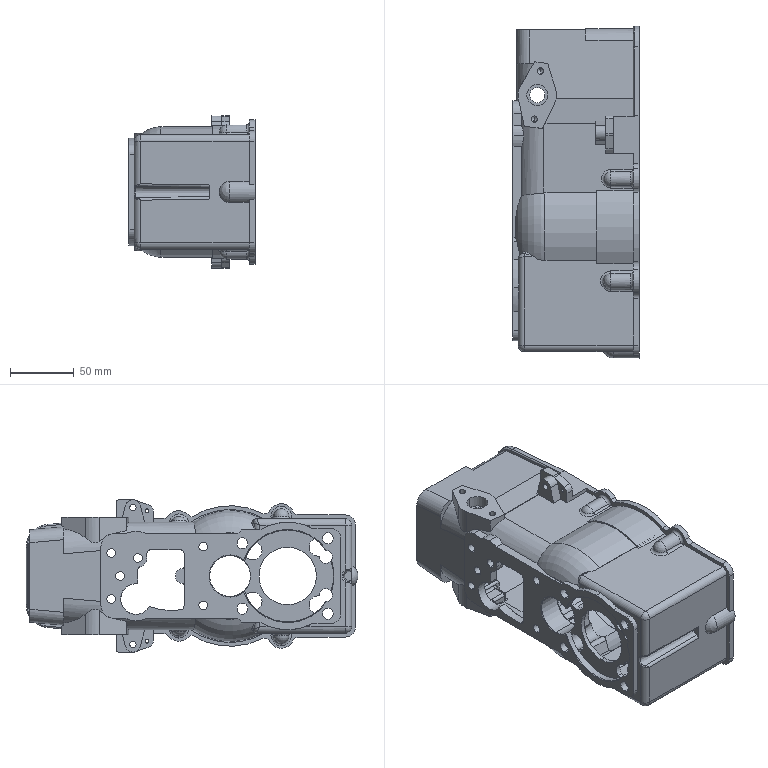Part | SolidWorks | features BaseBody 1 | 1 solid | 647 faces | box 98.5 x 259.5 x 119 mm | volume 419073 mm3 | cylinder 317 | plane 206 | spline 43 | torus 37 | cone 32 | sphere 12 | commonest cylinder face diameters 4 x50 10 x38 12 x28 5 x24 16 x13 4.9 x12